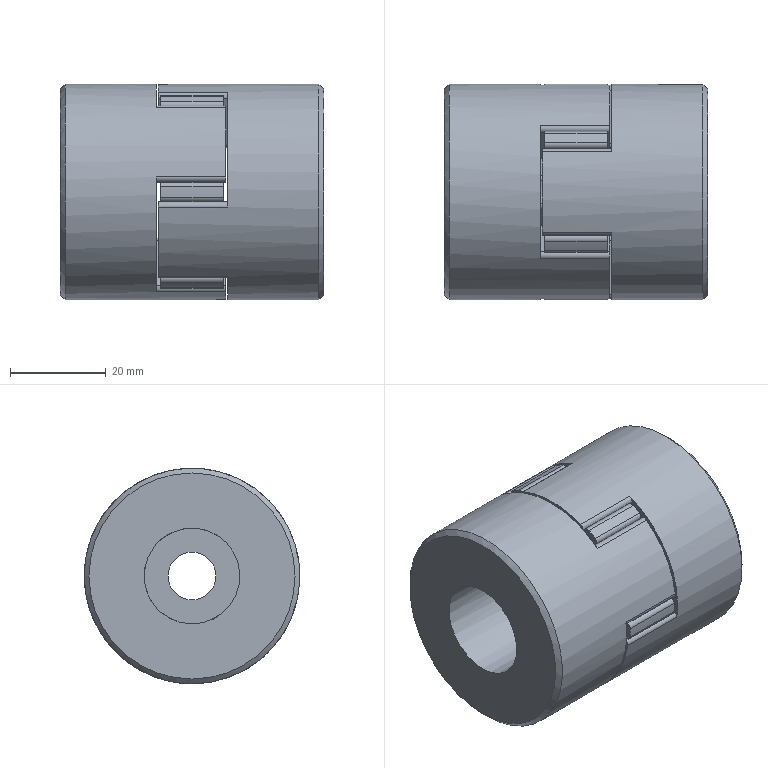Part | STEP file | YBQDJ-YB-23 | 1 solid | 119 faces | box 55 x 45 x 45 mm | volume 72571 mm3 | cylinder 65 | plane 52 | cone 2 | commonest cylinder face diameters 2 x48 45 x8 20 x7 10 x1 19 x1